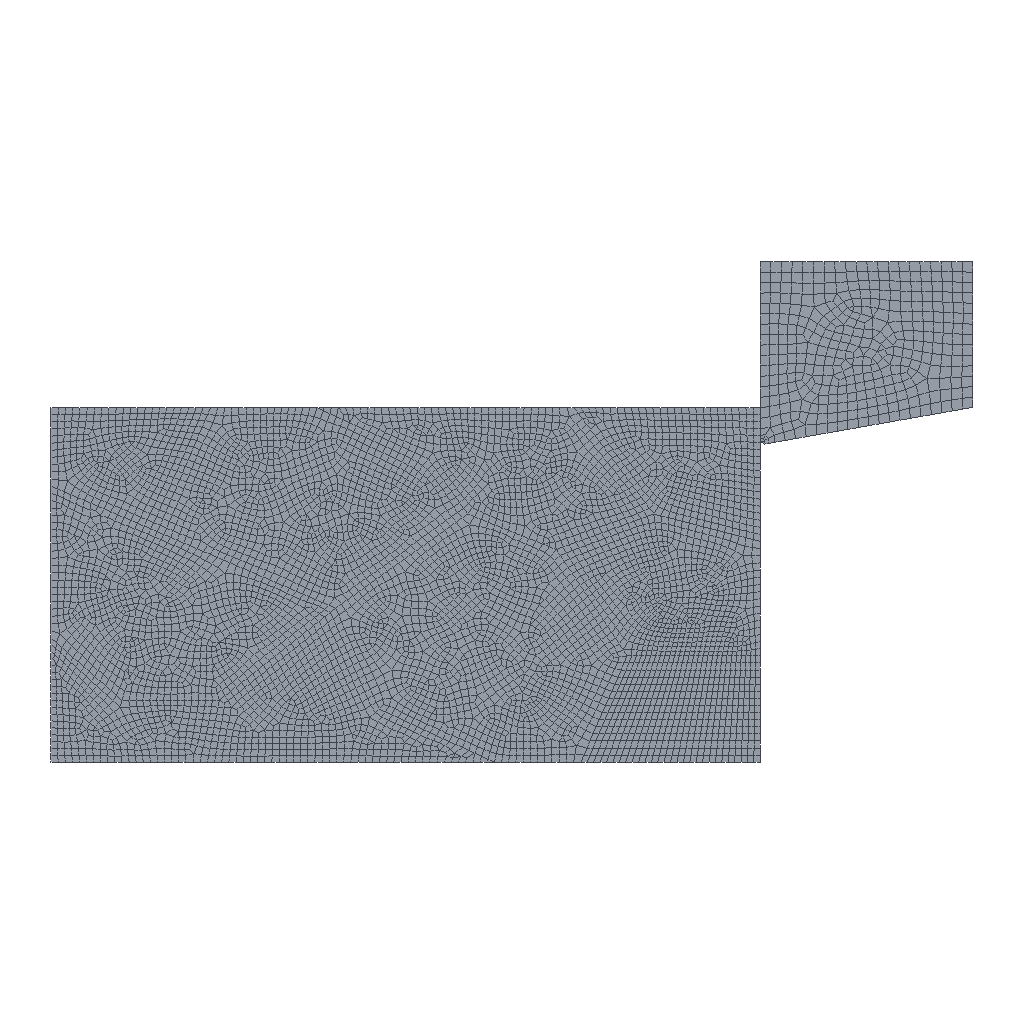Simulation study | abaqus
Set-up summary:
category,name,step,type,value,unit,region
solver,abaqus
solver,version,,,Abaqus/Explicit 3DEXPERIENCE R2017x
units,not stated in the deck,,not stated
analysis,deck,,transient,transient
load_step,Step-1,Step-1,transient
load_step,requested,,,1
mesh,nodes,,,6698
mesh,elements,,,6569
element_type,CPS3,,plane,122
element_type,CPS4R,,plane,6447
load,load commands in deck,,count,1
bc,support commands in deck,,count,4
material,TOOL,,in results
material,WORK,,in results
check,setup vs results,,match,"per instance, exact: element labels, types and connectivity; labels of the nodes the elements use; coordinates not compared"
Abaqus input file, long lists of numbers shortened:
*Heading
** Job name: Job-2 Model name: Model-1
** Generated by: Abaqus/CAE 2017
*Preprint, echo=NO, model=NO, history=NO, contact=NO
**
** PARTS
**
*Part, name=tool
*Node
      1,  3.31961091e-05, 0.01491
      2, 0.0001189, 0.01486
** (411 more lines like these left out)
*Element, type=CPS3
 1, 284, 252, 245
 2, 403, 303, 302
** (7 more lines like these left out)
*Element, type=CPS4R
 10, 393,  76,  59,   3
 11, 395,  76, 393, 394
** (368 more lines like these left out)
*Nset, nset=Set-1, generate
   1,  413,    1
*Elset, elset=Set-1, generate
   1,  379,    1
** Section: tool
*Solid Section, elset=Set-1, material=tool
,
*End Part
**
*Part, name=work
*Node
      1, 0.01625, -0.007
      2,  0.01494, -0.01
** (6283 more lines like these left out)
*Element, type=CPS4R
  1,   1,  25, 618, 106
  2,  25,  26, 619, 618
** (6075 more lines like these left out)
*Element, type=CPS3
421, 1127, 1172, 1124
422, 1249, 1165, 1236
** (111 more lines like these left out)
*Nset, nset=Set-1, generate
    1,  6285,     1
*Elset, elset=Set-1, generate
    1,  6190,     1
** Section: w
*Solid Section, elset=Set-1, material=work
,
*End Part
**
**
** ASSEMBLY
**
*Assembly, name=Assembly
**
*Instance, name=tool-1, part=tool
        0.02,    -0.01589,           0.
*End Instance
**
*Instance, name=work-1, part=work
*End Instance
**
*Node
      1, 0.026, 0.004113,           0.
*Nset, nset=Set-3, instance=work-1
   2,   3,   5,   8,   9,  11,  15,  39,  40,  41,  42,  43,  44,  45,  46,  47
  48,  49,  50,  51,  52,  53,  54,  55,  56,  57,  58,  59,  60,  61,  62,  63
** (7 more lines like these left out)
*Elset, elset=Set-3, instance=work-1
   15,   30,   45,   60,   75,   90,  105,  120,  135,  150,  165,  180,  195,  210,  225,  240
  255,  270,  285,  300,  315,  330,  345,  360,  375,  390,  405,  420,  427,  428,  429,  435
** (7 more lines like these left out)
*Nset, nset=Set-5
 1,
*Nset, nset=b_Set-1, instance=tool-1, generate
   1,  413,    1
*Elset, elset=b_Set-1, instance=tool-1, generate
   1,  379,    1
*Nset, nset=s_Set-4, instance=work-1
   10,   11,   12,   13,   14,   17,   18,   19,   20,   21,   22,   23,   24,  178,  179,  180
  181,  182,  183,  184,  185,  186,  187,  188,  189,  190,  191,  192,  233,  234,  235,  236
** (148 more lines like these left out)
*Elset, elset=s_Set-4, instance=work-1
 1588, 1589, 1590, 1591, 1592, 1593, 1594, 1595, 1596, 1597, 1598, 1599, 1600, 1601, 1602, 1603
 1604, 1605, 1606, 1607, 1608, 1609, 1610, 1611, 1612, 1613, 1614, 1615, 1616, 1617, 1618, 1619
** (142 more lines like these left out)
*Nset, nset=_PickedSet8, internal
 1,
*Elset, elset=_m_Surf-1_S2, internal, instance=tool-1
  9, 15, 19, 42, 43, 59, 62, 63, 65, 68
*Elset, elset=_m_Surf-1_S1, internal, instance=tool-1
  16,  17,  18,  23,  25,  69,  89,  90,  92,  94,  96, 102, 121, 377
*Elset, elset=_m_Surf-1_S3, internal, instance=tool-1
  10,  22,  71,  74,  80,  99, 104
*Elset, elset=_m_Surf-1_S4, internal, instance=tool-1
  30,  58,  60,  64,  66,  67,  70,  82,  83, 129
*Surface, type=ELEMENT, name=m_Surf-1
_m_Surf-1_S2, S2
_m_Surf-1_S1, S1
_m_Surf-1_S4, S4
_m_Surf-1_S3, S3
*Surface, type=NODE, name=s_Set-4_CNS_, internal
s_Set-4, 1.
** Constraint: Constraint-1
*Rigid Body, ref node=_PickedSet8, elset=b_Set-1
*End Assembly
**
** MATERIALS
**
*Material, name=tool
*Density
 7.8e-09,
*Elastic
210000., 0.3
*Material, name=work
*Damage Initiation, criterion=SHEAR
 0.001,0.,0.
*Damage Evolution, type=DISPLACEMENT
 1e-06,
*Density
 2e-09,
*Elastic
75400., 0.3
*Plastic
390.,   0.
420., 0.01
**
** INTERACTION PROPERTIES
**
*Surface Interaction, name=IntProp-1
*Friction
 0.15,
*Surface Behavior, pressure-overclosure=HARD
** ----------------------------------------------------------------
**
** STEP: Step-1
**
*Step, name=Step-1, nlgeom=YES
*Dynamic, Explicit
, 0.0001
*Bulk Viscosity
0.06, 1.2
** Mass Scaling: Semi-Automatic
**               Whole Model
*Fixed Mass Scaling, factor=500.
**
** BOUNDARY CONDITIONS
**
** Name: BC-1 Type: 对称/反对称/完全固定
*Boundary
Set-3, ENCASTRE
** Name: [REDACTED] : Velocity/Angular velocity
*Boundary, type=VELOCITY
Set-5, 1, 1, -200.
Set-5, 2, 2
Set-5, 6, 6
**
** INTERACTIONS
**
** Interaction: Int-1
*Contact Pair, interaction=IntProp-1, mechanical constraint=KINEMATIC, cpset=Int-1
m_Surf-1, s_Set-4_CNS_
**
** OUTPUT REQUESTS
**
*Restart, write, number interval=1, time marks=NO
**
** FIELD OUTPUT: F-Output-1
**
*Output, field, number interval=50
*Node Output
A, CF, RF, RM, RT, U, V
*Element Output, directions=YES
E, EVF, LE, MISES, MISESMAX, MISESONLY, PE, PEEQ, PEEQVAVG, PEVAVG, PRESSONLY, S, SSAVG, STATUS, SVAVG
*Contact Output
CDISP, CSTRESS
**
** HISTORY OUTPUT: H-Output-1
**
*Output, history, time interval=2e-09
*Node Output, nset=Set-5
RF1, RF2, RF3
*End Step
Results summary:
result,step,Step-1,completed,increments=335076 time=0.0001/0.0001
result,analysis,,,transient
result,last_loadstep,,,1
result,primary field,,,U
result,reaction total,,FX,0.4624,model units
result,reaction total,,FY,-0.04952,model units
result,reaction total,,FZ,0.0,model units